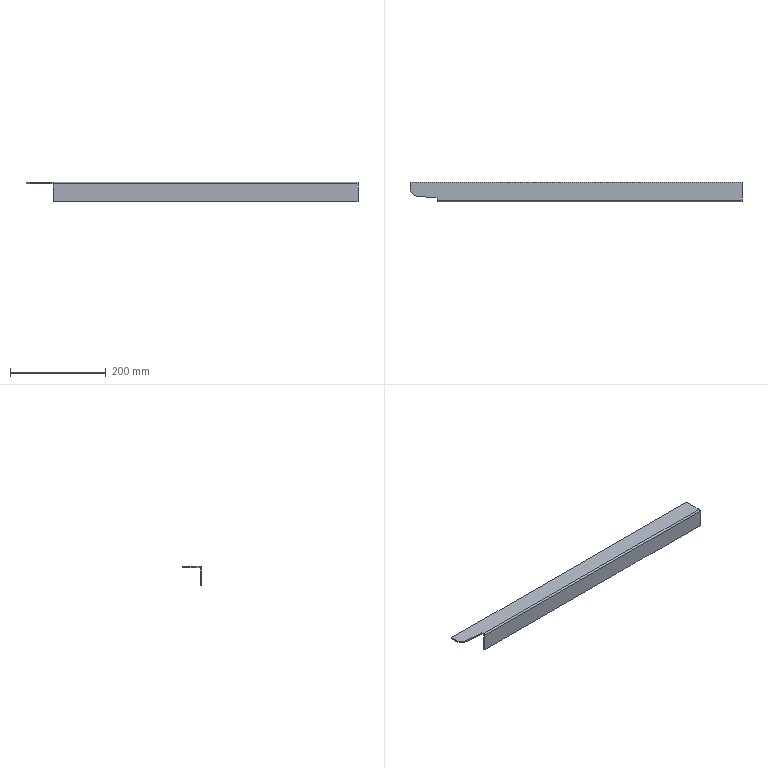Part | SolidWorks | 1 solid | 18 faces | box 693.5 x 40 x 40 mm | volume 150796 mm3 | plane 16 | cylinder 2 | commonest cylinder face diameters 0.2 x1 6.2 x1
STEP:
#1=CARTESIAN_POINT('',(-290.25,0.,-3.1));
#2=VERTEX_POINT('',#1);
#3=CARTESIAN_POINT('',(-290.25,0.,-40.));
#4=VERTEX_POINT('',#3);
#5=CARTESIAN_POINT('',(-290.25,0.,0.));
#6=DIRECTION('',(0.,0.,-1.));
#7=VECTOR('',#6,1000.);
#8=LINE('',#5,#7);
#9=EDGE_CURVE('',#2,#4,#8,.T.);
#10=ORIENTED_EDGE('',*,*,#9,.T.);
#11=CARTESIAN_POINT('',(346.75,0.,-40.));
#12=VERTEX_POINT('',#11);
#13=CARTESIAN_POINT('',(346.75,0.,-40.));
#14=DIRECTION('',(-1.,0.,0.));
#15=VECTOR('',#14,1000.);
#16=LINE('',#13,#15);
#17=EDGE_CURVE('',#12,#4,#16,.T.);
#18=ORIENTED_EDGE('',*,*,#17,.F.);
#19=CARTESIAN_POINT('',(346.75,0.,-3.1));
#20=VERTEX_POINT('',#19);
#21=CARTESIAN_POINT('',(346.75,0.,0.));
#22=DIRECTION('',(0.,0.,-1.));
#23=VECTOR('',#22,1000.);
#24=LINE('',#21,#23);
#25=EDGE_CURVE('',#20,#12,#24,.T.);
#26=ORIENTED_EDGE('',*,*,#25,.F.);
#27=CARTESIAN_POINT('',(346.75,0.,-3.1));
#28=DIRECTION('',(-1.,0.,0.));
#29=VECTOR('',#28,1000.);
#30=LINE('',#27,#29);
#31=EDGE_CURVE('',#20,#2,#30,.T.);
#32=ORIENTED_EDGE('',*,*,#31,.T.);
#33=EDGE_LOOP('',(#10,#18,#26,#32));
#34=FACE_OUTER_BOUND('',#33,.T.);
#35=CARTESIAN_POINT('',(346.75,0.,0.));
#36=DIRECTION('',(0.,1.,0.));
#37=DIRECTION('',(0.,0.,1.));
#38=AXIS2_PLACEMENT_3D('',#35,#36,#37);
#39=PLANE('',#38);
#40=ADVANCED_FACE('',(#34),#39,.F.);
#41=ORIENTED_EDGE('',*,*,#17,.T.);
#42=CARTESIAN_POINT('',(-290.25,3.,-40.));
#43=VERTEX_POINT('',#42);
#44=CARTESIAN_POINT('',(-290.25,3.,-40.));
#45=DIRECTION('',(0.,-1.,0.));
#46=VECTOR('',#45,1000.);
#47=LINE('',#44,#46);
#48=EDGE_CURVE('',#43,#4,#47,.T.);
#49=ORIENTED_EDGE('',*,*,#48,.F.);
#50=CARTESIAN_POINT('',(346.75,3.,-40.));
#51=VERTEX_POINT('',#50);
#52=CARTESIAN_POINT('',(346.75,3.,-40.));
#53=DIRECTION('',(-1.,0.,0.));
#54=VECTOR('',#53,1000.);
#55=LINE('',#52,#54);
#56=EDGE_CURVE('',#51,#43,#55,.T.);
#57=ORIENTED_EDGE('',*,*,#56,.F.);
#58=CARTESIAN_POINT('',(346.75,3.,-40.));
#59=DIRECTION('',(0.,-1.,0.));
#60=VECTOR('',#59,1000.);
#61=LINE('',#58,#60);
#62=EDGE_CURVE('',#51,#12,#61,.T.);
#63=ORIENTED_EDGE('',*,*,#62,.T.);
#64=EDGE_LOOP('',(#41,#49,#57,#63));
#65=FACE_OUTER_BOUND('',#64,.T.);
#66=CARTESIAN_POINT('',(346.75,3.,-40.));
#67=DIRECTION('',(0.,0.,-1.));
#68=DIRECTION('',(-1.,0.,0.));
#69=AXIS2_PLACEMENT_3D('',#66,#67,#68);
#70=PLANE('',#69);
#71=ADVANCED_FACE('',(#65),#70,.T.);
#72=ORIENTED_EDGE('',*,*,#56,.T.);
#73=CARTESIAN_POINT('',(-290.25,3.,-3.1));
#74=VERTEX_POINT('',#73);
#75=CARTESIAN_POINT('',(-290.25,3.,0.));
#76=DIRECTION('',(0.,0.,-1.));
#77=VECTOR('',#76,1000.);
#78=LINE('',#75,#77);
#79=EDGE_CURVE('',#74,#43,#78,.T.);
#80=ORIENTED_EDGE('',*,*,#79,.F.);
#81=CARTESIAN_POINT('',(346.75,3.,-3.1));
#82=VERTEX_POINT('',#81);
#83=CARTESIAN_POINT('',(346.75,3.,-3.1));
#84=DIRECTION('',(-1.,0.,0.));
#85=VECTOR('',#84,1000.);
#86=LINE('',#83,#85);
#87=EDGE_CURVE('',#82,#74,#86,.T.);
#88=ORIENTED_EDGE('',*,*,#87,.F.);
#89=CARTESIAN_POINT('',(346.75,3.,0.));
#90=DIRECTION('',(0.,0.,-1.));
#91=VECTOR('',#90,1000.);
#92=LINE('',#89,#91);
#93=EDGE_CURVE('',#82,#51,#92,.T.);
#94=ORIENTED_EDGE('',*,*,#93,.T.);
#95=EDGE_LOOP('',(#72,#80,#88,#94));
#96=FACE_OUTER_BOUND('',#95,.T.);
#97=CARTESIAN_POINT('',(346.75,3.,0.));
#98=DIRECTION('',(0.,1.,0.));
#99=DIRECTION('',(0.,0.,1.));
#100=AXIS2_PLACEMENT_3D('',#97,#98,#99);
#101=PLANE('',#100);
#102=ADVANCED_FACE('',(#96),#101,.T.);
#103=ORIENTED_EDGE('',*,*,#87,.T.);
#104=CARTESIAN_POINT('',(-290.25,3.1,-3.));
#105=VERTEX_POINT('',#104);
#106=CARTESIAN_POINT('',(-290.25,3.1,-3.1));
#107=DIRECTION('',(1.,0.,0.));
#108=DIRECTION('',(0.,0.,-1.));
#109=AXIS2_PLACEMENT_3D('',#106,#107,#108);
#110=CIRCLE('',#109,0.1);
#111=EDGE_CURVE('',#105,#74,#110,.T.);
#112=ORIENTED_EDGE('',*,*,#111,.F.);
#113=CARTESIAN_POINT('',(346.75,3.1,-3.));
#114=VERTEX_POINT('',#113);
#115=CARTESIAN_POINT('',(346.75,3.1,-3.));
#116=DIRECTION('',(-1.,0.,0.));
#117=VECTOR('',#116,1000.);
#118=LINE('',#115,#117);
#119=EDGE_CURVE('',#114,#105,#118,.T.);
#120=ORIENTED_EDGE('',*,*,#119,.F.);
#121=CARTESIAN_POINT('',(346.75,3.1,-3.1));
#122=DIRECTION('',(1.,0.,0.));
#123=DIRECTION('',(0.,0.,-1.));
#124=AXIS2_PLACEMENT_3D('',#121,#122,#123);
#125=CIRCLE('',#124,0.1);
#126=EDGE_CURVE('',#114,#82,#125,.T.);
#127=ORIENTED_EDGE('',*,*,#126,.T.);
#128=EDGE_LOOP('',(#103,#112,#120,#127));
#129=FACE_OUTER_BOUND('',#128,.T.);
#130=CARTESIAN_POINT('',(346.75,3.1,-3.1));
#131=DIRECTION('',(-1.,0.,0.));
#132=DIRECTION('',(0.,0.,1.));
#133=AXIS2_PLACEMENT_3D('',#130,#131,#132);
#134=CYLINDRICAL_SURFACE('',#133,0.1);
#135=ADVANCED_FACE('',(#129),#134,.F.);
#136=CARTESIAN_POINT('',(-337.795,12.028,-3.));
#137=VERTEX_POINT('',#136);
#138=CARTESIAN_POINT('',(-294.727,7.501,-3.));
#139=VERTEX_POINT('',#138);
#140=CARTESIAN_POINT('',(336.363,-58.829,-3.));
#141=DIRECTION('',(0.9945,-0.1045,0.));
#142=VECTOR('',#141,1000.);
#143=LINE('',#140,#142);
#144=EDGE_CURVE('',#137,#139,#143,.T.);
#145=ORIENTED_EDGE('',*,*,#144,.F.);
#146=CARTESIAN_POINT('',(-346.75,21.973,-3.));
#147=VERTEX_POINT('',#146);
#148=CARTESIAN_POINT('',(-45.209,-312.922,-3.));
#149=DIRECTION('',(0.6691,-0.7431,0.));
#150=VECTOR('',#149,1000.);
#151=LINE('',#148,#150);
#152=EDGE_CURVE('',#147,#137,#151,.T.);
#153=ORIENTED_EDGE('',*,*,#152,.F.);
#154=CARTESIAN_POINT('',(-346.75,40.,-3.));
#155=VERTEX_POINT('',#154);
#156=CARTESIAN_POINT('',(-346.75,40.,-3.));
#157=DIRECTION('',(0.,-1.,0.));
#158=VECTOR('',#157,1000.);
#159=LINE('',#156,#158);
#160=EDGE_CURVE('',#155,#147,#159,.T.);
#161=ORIENTED_EDGE('',*,*,#160,.F.);
#162=CARTESIAN_POINT('',(346.75,40.,-3.));
#163=VERTEX_POINT('',#162);
#164=CARTESIAN_POINT('',(346.75,40.,-3.));
#165=DIRECTION('',(-1.,0.,0.));
#166=VECTOR('',#165,1000.);
#167=LINE('',#164,#166);
#168=EDGE_CURVE('',#163,#155,#167,.T.);
#169=ORIENTED_EDGE('',*,*,#168,.F.);
#170=CARTESIAN_POINT('',(346.75,40.,-3.));
#171=DIRECTION('',(0.,-1.,0.));
#172=VECTOR('',#171,1000.);
#173=LINE('',#170,#172);
#174=EDGE_CURVE('',#163,#114,#173,.T.);
#175=ORIENTED_EDGE('',*,*,#174,.T.);
#176=ORIENTED_EDGE('',*,*,#119,.T.);
#177=CARTESIAN_POINT('',(-290.25,7.501,-3.));
#178=VERTEX_POINT('',#177);
#179=CARTESIAN_POINT('',(-290.25,40.,-3.));
#180=DIRECTION('',(0.,-1.,0.));
#181=VECTOR('',#180,1000.);
#182=LINE('',#179,#181);
#183=EDGE_CURVE('',#178,#105,#182,.T.);
#184=ORIENTED_EDGE('',*,*,#183,.F.);
#185=CARTESIAN_POINT('',(346.75,7.501,-3.));
#186=DIRECTION('',(1.,0.,0.));
#187=VECTOR('',#186,1000.);
#188=LINE('',#185,#187);
#189=EDGE_CURVE('',#139,#178,#188,.T.);
#190=ORIENTED_EDGE('',*,*,#189,.F.);
#191=EDGE_LOOP('',(#145,#153,#161,#169,#175,#176,#184,#190));
#192=FACE_OUTER_BOUND('',#191,.T.);
#193=CARTESIAN_POINT('',(346.75,40.,-3.));
#194=DIRECTION('',(0.,0.,-1.));
#195=DIRECTION('',(0.,1.,0.));
#196=AXIS2_PLACEMENT_3D('',#193,#194,#195);
#197=PLANE('',#196);
#198=ADVANCED_FACE('',(#192),#197,.T.);
#199=CARTESIAN_POINT('',(-346.75,21.973,0.));
#200=VERTEX_POINT('',#199);
#201=CARTESIAN_POINT('',(-337.795,12.028,0.));
#202=VERTEX_POINT('',#201);
#203=CARTESIAN_POINT('',(-45.209,-312.922,0.));
#204=DIRECTION('',(0.6691,-0.7431,0.));
#205=VECTOR('',#204,1000.);
#206=LINE('',#203,#205);
#207=EDGE_CURVE('',#200,#202,#206,.T.);
#208=ORIENTED_EDGE('',*,*,#207,.T.);
#209=CARTESIAN_POINT('',(-294.727,7.501,0.));
#210=VERTEX_POINT('',#209);
#211=CARTESIAN_POINT('',(336.363,-58.829,0.));
#212=DIRECTION('',(0.9945,-0.1045,0.));
#213=VECTOR('',#212,1000.);
#214=LINE('',#211,#213);
#215=EDGE_CURVE('',#202,#210,#214,.T.);
#216=ORIENTED_EDGE('',*,*,#215,.T.);
#217=CARTESIAN_POINT('',(-290.25,7.501,0.));
#218=VERTEX_POINT('',#217);
#219=CARTESIAN_POINT('',(346.75,7.501,0.));
#220=DIRECTION('',(1.,0.,0.));
#221=VECTOR('',#220,1000.);
#222=LINE('',#219,#221);
#223=EDGE_CURVE('',#210,#218,#222,.T.);
#224=ORIENTED_EDGE('',*,*,#223,.T.);
#225=CARTESIAN_POINT('',(-290.25,3.1,0.));
#226=VERTEX_POINT('',#225);
#227=CARTESIAN_POINT('',(-290.25,40.,0.));
#228=DIRECTION('',(0.,-1.,0.));
#229=VECTOR('',#228,1000.);
#230=LINE('',#227,#229);
#231=EDGE_CURVE('',#218,#226,#230,.T.);
#232=ORIENTED_EDGE('',*,*,#231,.T.);
#233=CARTESIAN_POINT('',(346.75,3.1,0.));
#234=VERTEX_POINT('',#233);
#235=CARTESIAN_POINT('',(346.75,3.1,0.));
#236=DIRECTION('',(-1.,0.,0.));
#237=VECTOR('',#236,1000.);
#238=LINE('',#235,#237);
#239=EDGE_CURVE('',#234,#226,#238,.T.);
#240=ORIENTED_EDGE('',*,*,#239,.F.);
#241=CARTESIAN_POINT('',(346.75,40.,0.));
#242=VERTEX_POINT('',#241);
#243=CARTESIAN_POINT('',(346.75,40.,0.));
#244=DIRECTION('',(0.,-1.,0.));
#245=VECTOR('',#244,1000.);
#246=LINE('',#243,#245);
#247=EDGE_CURVE('',#242,#234,#246,.T.);
#248=ORIENTED_EDGE('',*,*,#247,.F.);
#249=CARTESIAN_POINT('',(-346.75,40.,0.));
#250=VERTEX_POINT('',#249);
#251=CARTESIAN_POINT('',(346.75,40.,0.));
#252=DIRECTION('',(-1.,0.,0.));
#253=VECTOR('',#252,1000.);
#254=LINE('',#251,#253);
#255=EDGE_CURVE('',#242,#250,#254,.T.);
#256=ORIENTED_EDGE('',*,*,#255,.T.);
#257=CARTESIAN_POINT('',(-346.75,40.,0.));
#258=DIRECTION('',(0.,-1.,0.));
#259=VECTOR('',#258,1000.);
#260=LINE('',#257,#259);
#261=EDGE_CURVE('',#250,#200,#260,.T.);
#262=ORIENTED_EDGE('',*,*,#261,.T.);
#263=EDGE_LOOP('',(#208,#216,#224,#232,#240,#248,#256,#262));
#264=FACE_OUTER_BOUND('',#263,.T.);
#265=CARTESIAN_POINT('',(346.75,40.,0.));
#266=DIRECTION('',(0.,0.,-1.));
#267=DIRECTION('',(0.,1.,0.));
#268=AXIS2_PLACEMENT_3D('',#265,#266,#267);
#269=PLANE('',#268);
#270=ADVANCED_FACE('',(#264),#269,.F.);
#271=CARTESIAN_POINT('',(-290.25,3.1,-3.1));
#272=DIRECTION('',(1.,0.,0.));
#273=DIRECTION('',(0.,0.,1.));
#274=AXIS2_PLACEMENT_3D('',#271,#272,#273);
#275=CIRCLE('',#274,3.1);
#276=EDGE_CURVE('',#226,#2,#275,.T.);
#277=ORIENTED_EDGE('',*,*,#276,.T.);
#278=ORIENTED_EDGE('',*,*,#31,.F.);
#279=CARTESIAN_POINT('',(346.75,3.1,-3.1));
#280=DIRECTION('',(1.,0.,0.));
#281=DIRECTION('',(0.,0.,1.));
#282=AXIS2_PLACEMENT_3D('',#279,#280,#281);
#283=CIRCLE('',#282,3.1);
#284=EDGE_CURVE('',#234,#20,#283,.T.);
#285=ORIENTED_EDGE('',*,*,#284,.F.);
#286=ORIENTED_EDGE('',*,*,#239,.T.);
#287=EDGE_LOOP('',(#277,#278,#285,#286));
#288=FACE_OUTER_BOUND('',#287,.T.);
#289=CARTESIAN_POINT('',(346.75,3.1,-3.1));
#290=DIRECTION('',(-1.,0.,0.));
#291=DIRECTION('',(0.,0.,1.));
#292=AXIS2_PLACEMENT_3D('',#289,#290,#291);
#293=CYLINDRICAL_SURFACE('',#292,3.1);
#294=ADVANCED_FACE('',(#288),#293,.T.);
#295=CARTESIAN_POINT('',(346.75,3.1,0.));
#296=DIRECTION('',(0.,0.,-1.));
#297=VECTOR('',#296,1000.);
#298=LINE('',#295,#297);
#299=EDGE_CURVE('',#234,#114,#298,.T.);
#300=ORIENTED_EDGE('',*,*,#299,.F.);
#301=ORIENTED_EDGE('',*,*,#284,.T.);
#302=CARTESIAN_POINT('',(346.75,3.,-3.1));
#303=DIRECTION('',(0.,-1.,0.));
#304=VECTOR('',#303,1000.);
#305=LINE('',#302,#304);
#306=EDGE_CURVE('',#82,#20,#305,.T.);
#307=ORIENTED_EDGE('',*,*,#306,.F.);
#308=ORIENTED_EDGE('',*,*,#126,.F.);
#309=EDGE_LOOP('',(#300,#301,#307,#308));
#310=FACE_OUTER_BOUND('',#309,.T.);
#311=CARTESIAN_POINT('',(346.75,3.1,0.));
#312=DIRECTION('',(1.,0.,0.));
#313=DIRECTION('',(0.,0.,-1.));
#314=AXIS2_PLACEMENT_3D('',#311,#312,#313);
#315=PLANE('',#314);
#316=ADVANCED_FACE('',(#310),#315,.T.);
#317=ORIENTED_EDGE('',*,*,#247,.T.);
#318=ORIENTED_EDGE('',*,*,#299,.T.);
#319=ORIENTED_EDGE('',*,*,#174,.F.);
#320=CARTESIAN_POINT('',(346.75,40.,0.));
#321=DIRECTION('',(0.,0.,-1.));
#322=VECTOR('',#321,1000.);
#323=LINE('',#320,#322);
#324=EDGE_CURVE('',#242,#163,#323,.T.);
#325=ORIENTED_EDGE('',*,*,#324,.F.);
#326=EDGE_LOOP('',(#317,#318,#319,#325));
#327=FACE_OUTER_BOUND('',#326,.T.);
#328=CARTESIAN_POINT('',(346.75,3.,-3.1));
#329=DIRECTION('',(1.,0.,0.));
#330=DIRECTION('',(0.,0.,-1.));
#331=AXIS2_PLACEMENT_3D('',#328,#329,#330);
#332=PLANE('',#331);
#333=ADVANCED_FACE('',(#327),#332,.T.);
#334=CARTESIAN_POINT('',(-346.75,40.,0.));
#335=DIRECTION('',(0.,0.,-1.));
#336=VECTOR('',#335,1000.);
#337=LINE('',#334,#336);
#338=EDGE_CURVE('',#250,#155,#337,.T.);
#339=ORIENTED_EDGE('',*,*,#338,.F.);
#340=ORIENTED_EDGE('',*,*,#255,.F.);
#341=ORIENTED_EDGE('',*,*,#324,.T.);
#342=ORIENTED_EDGE('',*,*,#168,.T.);
#343=EDGE_LOOP('',(#339,#340,#341,#342));
#344=FACE_OUTER_BOUND('',#343,.T.);
#345=CARTESIAN_POINT('',(346.75,40.,0.));
#346=DIRECTION('',(0.,1.,0.));
#347=DIRECTION('',(0.,0.,1.));
#348=AXIS2_PLACEMENT_3D('',#345,#346,#347);
#349=PLANE('',#348);
#350=ADVANCED_FACE('',(#344),#349,.T.);
#351=ORIENTED_EDGE('',*,*,#25,.T.);
#352=ORIENTED_EDGE('',*,*,#62,.F.);
#353=ORIENTED_EDGE('',*,*,#93,.F.);
#354=ORIENTED_EDGE('',*,*,#306,.T.);
#355=EDGE_LOOP('',(#351,#352,#353,#354));
#356=FACE_OUTER_BOUND('',#355,.T.);
#357=CARTESIAN_POINT('',(346.75,3.1,-3.1));
#358=DIRECTION('',(1.,0.,0.));
#359=DIRECTION('',(0.,0.,-1.));
#360=AXIS2_PLACEMENT_3D('',#357,#358,#359);
#361=PLANE('',#360);
#362=ADVANCED_FACE('',(#356),#361,.T.);
#363=CARTESIAN_POINT('',(-346.75,21.973,-3.));
#364=DIRECTION('',(0.,0.,1.));
#365=VECTOR('',#364,1000.);
#366=LINE('',#363,#365);
#367=EDGE_CURVE('',#147,#200,#366,.T.);
#368=ORIENTED_EDGE('',*,*,#367,.T.);
#369=ORIENTED_EDGE('',*,*,#261,.F.);
#370=ORIENTED_EDGE('',*,*,#338,.T.);
#371=ORIENTED_EDGE('',*,*,#160,.T.);
#372=EDGE_LOOP('',(#368,#369,#370,#371));
#373=FACE_OUTER_BOUND('',#372,.T.);
#374=CARTESIAN_POINT('',(-346.75,3.1,-3.1));
#375=DIRECTION('',(1.,0.,0.));
#376=DIRECTION('',(0.,0.,-1.));
#377=AXIS2_PLACEMENT_3D('',#374,#375,#376);
#378=PLANE('',#377);
#379=ADVANCED_FACE('',(#373),#378,.F.);
#380=ORIENTED_EDGE('',*,*,#79,.T.);
#381=ORIENTED_EDGE('',*,*,#48,.T.);
#382=ORIENTED_EDGE('',*,*,#9,.F.);
#383=CARTESIAN_POINT('',(-290.25,3.,-3.1));
#384=DIRECTION('',(0.,-1.,0.));
#385=VECTOR('',#384,1000.);
#386=LINE('',#383,#385);
#387=EDGE_CURVE('',#74,#2,#386,.T.);
#388=ORIENTED_EDGE('',*,*,#387,.F.);
#389=EDGE_LOOP('',(#380,#381,#382,#388));
#390=FACE_OUTER_BOUND('',#389,.T.);
#391=CARTESIAN_POINT('',(-290.25,3.,0.));
#392=DIRECTION('',(1.,0.,0.));
#393=DIRECTION('',(0.,0.,-1.));
#394=AXIS2_PLACEMENT_3D('',#391,#392,#393);
#395=PLANE('',#394);
#396=ADVANCED_FACE('',(#390),#395,.F.);
#397=ORIENTED_EDGE('',*,*,#367,.F.);
#398=ORIENTED_EDGE('',*,*,#152,.T.);
#399=CARTESIAN_POINT('',(-337.795,12.028,-3.));
#400=DIRECTION('',(0.,0.,1.));
#401=VECTOR('',#400,1000.);
#402=LINE('',#399,#401);
#403=EDGE_CURVE('',#137,#202,#402,.T.);
#404=ORIENTED_EDGE('',*,*,#403,.T.);
#405=ORIENTED_EDGE('',*,*,#207,.F.);
#406=EDGE_LOOP('',(#397,#398,#404,#405));
#407=FACE_OUTER_BOUND('',#406,.T.);
#408=CARTESIAN_POINT('',(-45.209,-312.922,-3.));
#409=DIRECTION('',(0.7431,0.6691,0.));
#410=DIRECTION('',(0.6691,-0.7431,0.));
#411=AXIS2_PLACEMENT_3D('',#408,#409,#410);
#412=PLANE('',#411);
#413=ADVANCED_FACE('',(#407),#412,.F.);
#414=ORIENTED_EDGE('',*,*,#403,.F.);
#415=ORIENTED_EDGE('',*,*,#144,.T.);
#416=CARTESIAN_POINT('',(-294.727,7.501,-3.));
#417=DIRECTION('',(0.,0.,1.));
#418=VECTOR('',#417,1000.);
#419=LINE('',#416,#418);
#420=EDGE_CURVE('',#139,#210,#419,.T.);
#421=ORIENTED_EDGE('',*,*,#420,.T.);
#422=ORIENTED_EDGE('',*,*,#215,.F.);
#423=EDGE_LOOP('',(#414,#415,#421,#422));
#424=FACE_OUTER_BOUND('',#423,.T.);
#425=CARTESIAN_POINT('',(336.363,-58.829,-3.));
#426=DIRECTION('',(0.1045,0.9945,0.));
#427=DIRECTION('',(0.9945,-0.1045,0.));
#428=AXIS2_PLACEMENT_3D('',#425,#426,#427);
#429=PLANE('',#428);
#430=ADVANCED_FACE('',(#424),#429,.F.);
#431=ORIENTED_EDGE('',*,*,#420,.F.);
#432=ORIENTED_EDGE('',*,*,#189,.T.);
#433=CARTESIAN_POINT('',(-290.25,7.501,-3.));
#434=DIRECTION('',(0.,0.,1.));
#435=VECTOR('',#434,1000.);
#436=LINE('',#433,#435);
#437=EDGE_CURVE('',#178,#218,#436,.T.);
#438=ORIENTED_EDGE('',*,*,#437,.T.);
#439=ORIENTED_EDGE('',*,*,#223,.F.);
#440=EDGE_LOOP('',(#431,#432,#438,#439));
#441=FACE_OUTER_BOUND('',#440,.T.);
#442=CARTESIAN_POINT('',(346.75,7.501,-3.));
#443=DIRECTION('',(0.,1.,0.));
#444=DIRECTION('',(1.,0.,0.));
#445=AXIS2_PLACEMENT_3D('',#442,#443,#444);
#446=PLANE('',#445);
#447=ADVANCED_FACE('',(#441),#446,.F.);
#448=ORIENTED_EDGE('',*,*,#183,.T.);
#449=CARTESIAN_POINT('',(-290.25,3.1,-3.));
#450=DIRECTION('',(0.,0.,1.));
#451=VECTOR('',#450,1000.);
#452=LINE('',#449,#451);
#453=EDGE_CURVE('',#105,#226,#452,.T.);
#454=ORIENTED_EDGE('',*,*,#453,.T.);
#455=ORIENTED_EDGE('',*,*,#231,.F.);
#456=ORIENTED_EDGE('',*,*,#437,.F.);
#457=EDGE_LOOP('',(#448,#454,#455,#456));
#458=FACE_OUTER_BOUND('',#457,.T.);
#459=CARTESIAN_POINT('',(-290.25,40.,-3.));
#460=DIRECTION('',(1.,0.,0.));
#461=DIRECTION('',(0.,-1.,0.));
#462=AXIS2_PLACEMENT_3D('',#459,#460,#461);
#463=PLANE('',#462);
#464=ADVANCED_FACE('',(#458),#463,.F.);
#465=ORIENTED_EDGE('',*,*,#111,.T.);
#466=ORIENTED_EDGE('',*,*,#387,.T.);
#467=ORIENTED_EDGE('',*,*,#276,.F.);
#468=ORIENTED_EDGE('',*,*,#453,.F.);
#469=EDGE_LOOP('',(#465,#466,#467,#468));
#470=FACE_OUTER_BOUND('',#469,.T.);
#471=CARTESIAN_POINT('',(-290.25,3.1,-3.1));
#472=DIRECTION('',(-1.,0.,0.));
#473=DIRECTION('',(0.,0.,1.));
#474=AXIS2_PLACEMENT_3D('',#471,#472,#473);
#475=PLANE('',#474);
#476=ADVANCED_FACE('',(#470),#475,.T.);
#477=CLOSED_SHELL('',(#40,#71,#102,#135,#198,#270,#294,#316,#333,#350,#362,#379,#396,#413,#430,#447,#464,#476));
#478=MANIFOLD_SOLID_BREP('',#477);
#479=CARTESIAN_POINT('',(0.,0.,0.));
#480=DIRECTION('',(0.,0.,1.));
#481=DIRECTION('',(1.,0.,0.));
#482=AXIS2_PLACEMENT_3D('',#479,#480,#481);
#483=(LENGTH_UNIT()NAMED_UNIT(*)SI_UNIT(.MILLI.,.METRE.));
#484=UNCERTAINTY_MEASURE_WITH_UNIT(LENGTH_MEASURE(0.00001),#483,'','');
#485=(NAMED_UNIT(*)PLANE_ANGLE_UNIT()SI_UNIT($,.RADIAN.));
#486=(NAMED_UNIT(*)SI_UNIT($,.STERADIAN.)SOLID_ANGLE_UNIT());
#487=(GEOMETRIC_REPRESENTATION_CONTEXT(3)GLOBAL_UNCERTAINTY_ASSIGNED_CONTEXT((#484))GLOBAL_UNIT_ASSIGNED_CONTEXT((#483,#485,#486))REPRESENTATION_CONTEXT('',''));
#488=ADVANCED_BREP_SHAPE_REPRESENTATION('',(#478,#482),#487);